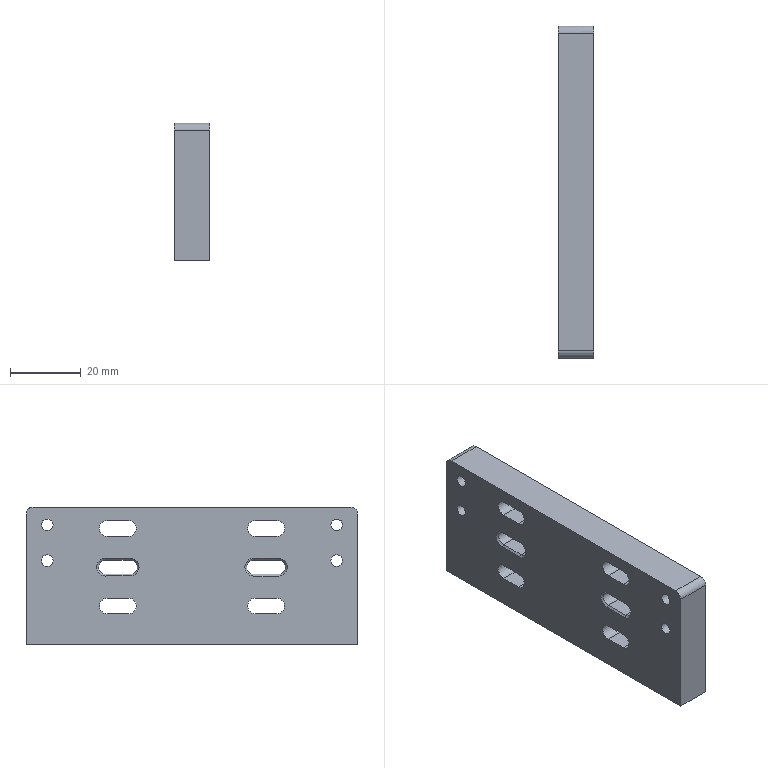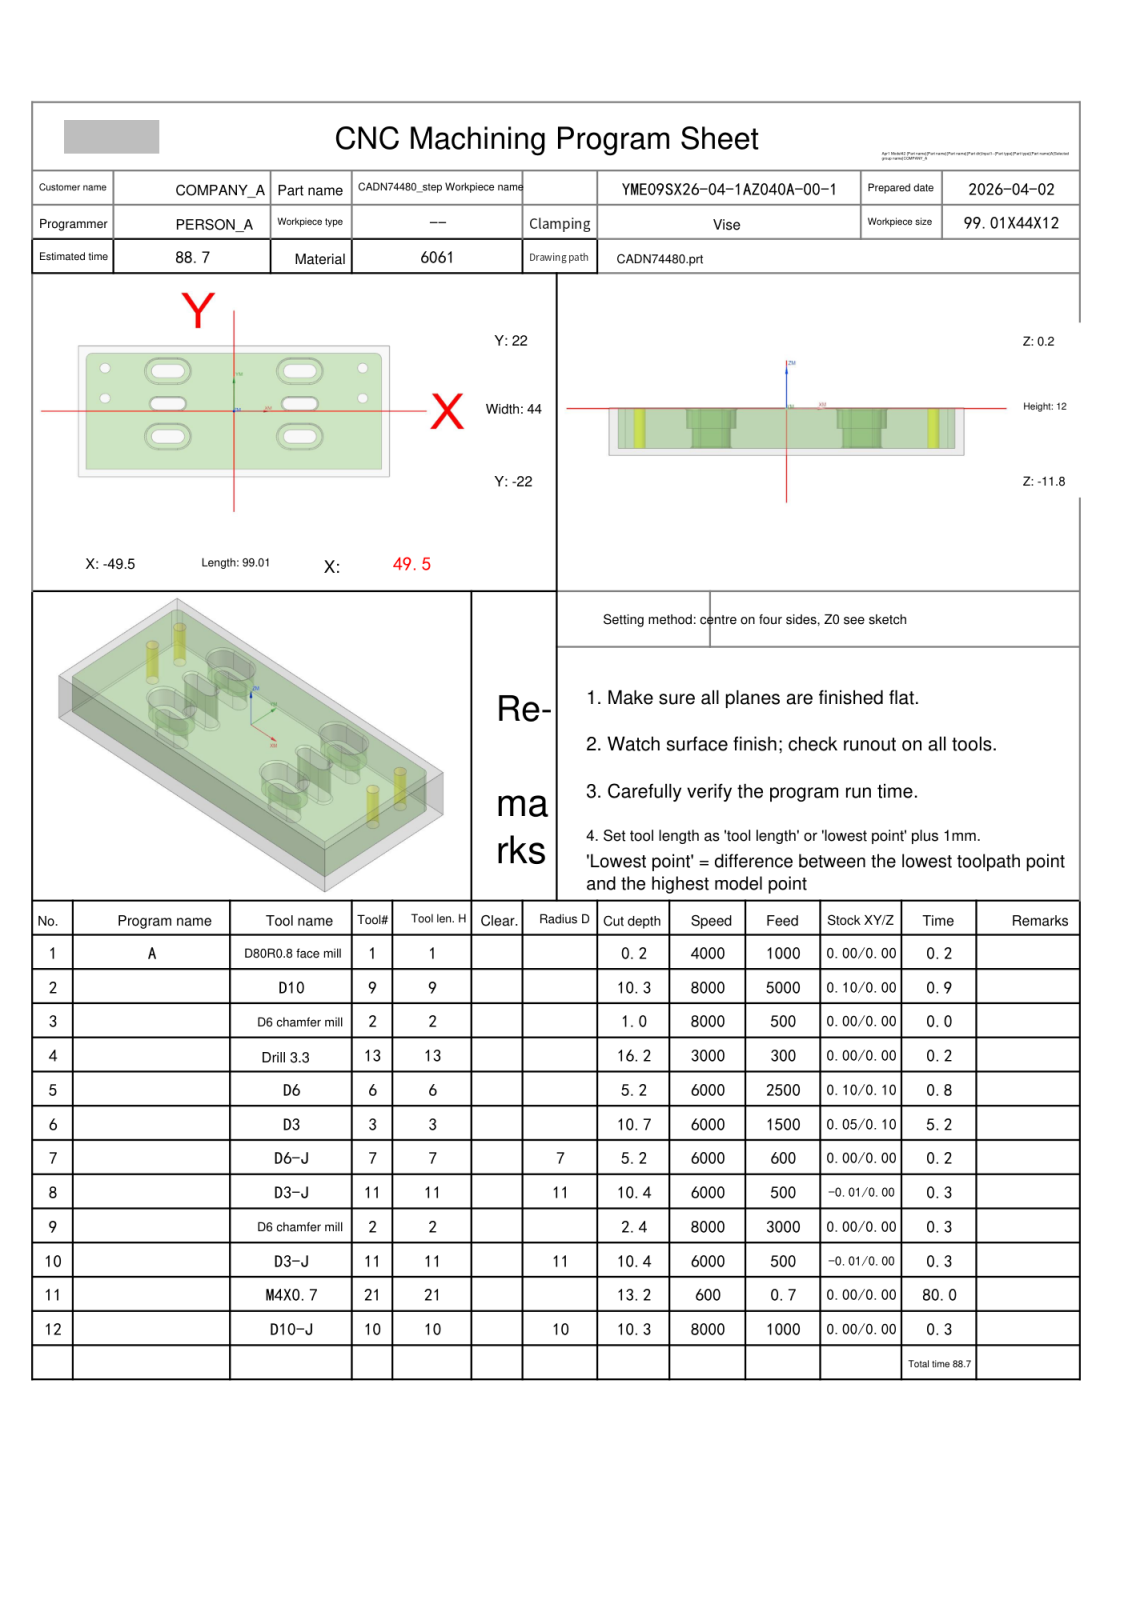NC program | NX | posted by the shop | part box 10.067 x 94 x 39 mm
Lines 938 to 1774 of 4590:
N6 T03 M06
(D3  D=3. R=0. H=03 ce=0.05 di=0.10)
G00 G90 G54 X21.004 Y-9.2 M03 S6000
G43 H03 Z20.
M08
Z-4.5
G01 X24.004 Z-4.518 F1500.
G03 X24.704 Y-8.5 Z-4.525 I0.0 J.7
X24.004 Y-7.8 Z-4.532 I-.7 J0.0
G01 X18.004 Z-4.568
G03 X17.304 Y-8.5 Z-4.575 I0.0 J-.7
X18.004 Y-9.2 Z-4.582 I.7 J0.0
G01 X24.004 Z-4.618
G03 X24.704 Y-8.5 Z-4.625 I0.0 J.7
X24.004 Y-7.8 Z-4.632 I-.7 J0.0
G01 X18.004 Z-4.668
G03 X17.304 Y-8.5 Z-4.675 I0.0 J-.7
X18.004 Y-9.2 Z-4.682 I.7 J0.0
G01 X24.004 Z-4.718
G03 X24.704 Y-8.5 Z-4.725 I0.0 J.7
X24.004 Y-7.8 Z-4.732 I-.7 J0.0
G01 X18.004 Z-4.768
G03 X17.304 Y-8.5 Z-4.775 I0.0 J-.7
X18.004 Y-9.2 Z-4.782 I.7 J0.0
G01 X24.004 Z-4.818
G03 X24.704 Y-8.5 Z-4.825 I0.0 J.7
X24.004 Y-7.8 Z-4.832 I-.7 J0.0
G01 X18.004 Z-4.868
G03 X17.304 Y-8.5 Z-4.875 I0.0 J-.7
X18.004 Y-9.2 Z-4.882 I.7 J0.0
G01 X24.004 Z-4.918
G03 X24.704 Y-8.5 Z-4.925 I0.0 J.7
X24.004 Y-7.8 Z-4.932 I-.7 J0.0
G01 X18.004 Z-4.968
G03 X17.304 Y-8.5 Z-4.975 I0.0 J-.7
X18.004 Y-9.2 Z-4.982 I.7 J0.0
G01 X24.004 Z-5.018
G03 X24.704 Y-8.5 Z-5.025 I0.0 J.7
X24.004 Y-7.8 Z-5.032 I-.7 J0.0
G01 X18.004 Z-5.068
G03 X17.304 Y-8.5 Z-5.075 I0.0 J-.7
X18.004 Y-9.2 Z-5.082 I.7 J0.0
G01 X24.004 Z-5.118
G03 X24.704 Y-8.5 Z-5.125 I0.0 J.7
X24.004 Y-7.8 Z-5.132 I-.7 J0.0
G01 X18.004 Z-5.168
G03 X17.304 Y-8.5 Z-5.175 I0.0 J-.7
X18.004 Y-9.2 Z-5.182 I.7 J0.0
G01 X24.004 Z-5.218
G03 X24.704 Y-8.5 Z-5.225 I0.0 J.7
X24.004 Y-7.8 Z-5.232 I-.7 J0.0
G01 X18.004 Z-5.268
G03 X17.304 Y-8.5 Z-5.275 I0.0 J-.7
X18.004 Y-9.2 Z-5.282 I.7 J0.0
G01 X24.004 Z-5.318
G03 X24.704 Y-8.5 Z-5.325 I0.0 J.7
X24.004 Y-7.8 Z-5.332 I-.7 J0.0
G01 X18.004 Z-5.368
G03 X17.304 Y-8.5 Z-5.375 I0.0 J-.7
X18.004 Y-9.2 Z-5.382 I.7 J0.0
G01 X24.004 Z-5.418
G03 X24.704 Y-8.5 Z-5.425 I0.0 J.7
X24.004 Y-7.8 Z-5.432 I-.7 J0.0
G01 X18.004 Z-5.468
G03 X17.304 Y-8.5 Z-5.475 I0.0 J-.7
X18.004 Y-9.2 Z-5.482 I.7 J0.0
G01 X24.004 Z-5.518
G03 X24.704 Y-8.5 Z-5.525 I0.0 J.7
X24.004 Y-7.8 Z-5.532 I-.7 J0.0
G01 X18.004 Z-5.568
G03 X17.304 Y-8.5 Z-5.575 I0.0 J-.7
X18.004 Y-9.2 Z-5.582 I.7 J0.0
G01 X24.004 Z-5.618
G03 X24.704 Y-8.5 Z-5.625 I0.0 J.7
X24.004 Y-7.8 Z-5.632 I-.7 J0.0
G01 X18.004 Z-5.668
G03 X17.304 Y-8.5 Z-5.675 I0.0 J-.7
X18.004 Y-9.2 Z-5.682 I.7 J0.0
G01 X24.004 Z-5.718
G03 X24.704 Y-8.5 Z-5.725 I0.0 J.7
X24.004 Y-7.8 Z-5.732 I-.7 J0.0
G01 X18.004 Z-5.768
G03 X17.304 Y-8.5 Z-5.775 I0.0 J-.7
X18.004 Y-9.2 Z-5.782 I.7 J0.0
G01 X24.004 Z-5.818
G03 X24.704 Y-8.5 Z-5.825 I0.0 J.7
X24.004 Y-7.8 Z-5.832 I-.7 J0.0
G01 X18.004 Z-5.868
G03 X17.304 Y-8.5 Z-5.875 I0.0 J-.7
X18.004 Y-9.2 Z-5.882 I.7 J0.0
G01 X24.004 Z-5.918
G03 X24.704 Y-8.5 Z-5.925 I0.0 J.7
X24.004 Y-7.8 Z-5.932 I-.7 J0.0
G01 X18.004 Z-5.968
G03 X17.304 Y-8.5 Z-5.975 I0.0 J-.7
X18.004 Y-9.2 Z-5.982 I.7 J0.0
G01 X24.004 Z-6.018
G03 X24.704 Y-8.5 Z-6.025 I0.0 J.7
X24.004 Y-7.8 Z-6.032 I-.7 J0.0
G01 X18.004 Z-6.068
G03 X17.304 Y-8.5 Z-6.075 I0.0 J-.7
X18.004 Y-9.2 Z-6.082 I.7 J0.0
G01 X24.004 Z-6.118
G03 X24.704 Y-8.5 Z-6.125 I0.0 J.7
X24.004 Y-7.8 Z-6.132 I-.7 J0.0
G01 X18.004 Z-6.168
G03 X17.304 Y-8.5 Z-6.175 I0.0 J-.7
X18.004 Y-9.2 Z-6.182 I.7 J0.0
G01 X24.004 Z-6.218
G03 X24.704 Y-8.5 Z-6.225 I0.0 J.7
X24.004 Y-7.8 Z-6.232 I-.7 J0.0
G01 X18.004 Z-6.268
G03 X17.304 Y-8.5 Z-6.275 I0.0 J-.7
X18.004 Y-9.2 Z-6.282 I.7 J0.0
G01 X24.004 Z-6.318
G03 X24.704 Y-8.5 Z-6.325 I0.0 J.7
X24.004 Y-7.8 Z-6.332 I-.7 J0.0
G01 X18.004 Z-6.368
G03 X17.304 Y-8.5 Z-6.375 I0.0 J-.7
X18.004 Y-9.2 Z-6.382 I.7 J0.0
G01 X24.004 Z-6.418
G03 X24.704 Y-8.5 Z-6.425 I0.0 J.7
X24.004 Y-7.8 Z-6.432 I-.7 J0.0
G01 X18.004 Z-6.468
G03 X17.304 Y-8.5 Z-6.475 I0.0 J-.7
X18.004 Y-9.2 Z-6.482 I.7 J0.0
G01 X24.004 Z-6.518
G03 X24.704 Y-8.5 Z-6.525 I0.0 J.7
X24.004 Y-7.8 Z-6.532 I-.7 J0.0
G01 X18.004 Z-6.568
G03 X17.304 Y-8.5 Z-6.575 I0.0 J-.7
X18.004 Y-9.2 Z-6.582 I.7 J0.0
G01 X24.004 Z-6.618
G03 X24.704 Y-8.5 Z-6.625 I0.0 J.7
X24.004 Y-7.8 Z-6.632 I-.7 J0.0
G01 X18.004 Z-6.668
G03 X17.304 Y-8.5 Z-6.675 I0.0 J-.7
X18.004 Y-9.2 Z-6.682 I.7 J0.0
G01 X24.004 Z-6.718
G03 X24.704 Y-8.5 Z-6.725 I0.0 J.7
X24.004 Y-7.8 Z-6.732 I-.7 J0.0
G01 X18.004 Z-6.768
G03 X17.304 Y-8.5 Z-6.775 I0.0 J-.7
X18.004 Y-9.2 Z-6.782 I.7 J0.0
G01 X24.004 Z-6.818
G03 X24.704 Y-8.5 Z-6.825 I0.0 J.7
X24.004 Y-7.8 Z-6.832 I-.7 J0.0
G01 X18.004 Z-6.868
G03 X17.304 Y-8.5 Z-6.875 I0.0 J-.7
X18.004 Y-9.2 Z-6.882 I.7 J0.0
G01 X24.004 Z-6.918
G03 X24.704 Y-8.5 Z-6.925 I0.0 J.7
X24.004 Y-7.8 Z-6.932 I-.7 J0.0
G01 X18.004 Z-6.968
G03 X17.304 Y-8.5 Z-6.975 I0.0 J-.7
X18.004 Y-9.2 Z-6.982 I.7 J0.0
G01 X24.004 Z-7.018
G03 X24.704 Y-8.5 Z-7.025 I0.0 J.7
X24.004 Y-7.8 Z-7.032 I-.7 J0.0
G01 X18.004 Z-7.068
G03 X17.304 Y-8.5 Z-7.075 I0.0 J-.7
X18.004 Y-9.2 Z-7.082 I.7 J0.0
G01 X24.004 Z-7.118
G03 X24.704 Y-8.5 Z-7.125 I0.0 J.7
X24.004 Y-7.8 Z-7.132 I-.7 J0.0
G01 X18.004 Z-7.168
G03 X17.304 Y-8.5 Z-7.175 I0.0 J-.7
X18.004 Y-9.2 Z-7.182 I.7 J0.0
G01 X24.004 Z-7.218
G03 X24.704 Y-8.5 Z-7.225 I0.0 J.7
X24.004 Y-7.8 Z-7.232 I-.7 J0.0
G01 X18.004 Z-7.268
G03 X17.304 Y-8.5 Z-7.275 I0.0 J-.7
X18.004 Y-9.2 Z-7.282 I.7 J0.0
G01 X24.004 Z-7.318
G03 X24.704 Y-8.5 Z-7.325 I0.0 J.7
X24.004 Y-7.8 Z-7.332 I-.7 J0.0
G01 X18.004 Z-7.368
G03 X17.304 Y-8.5 Z-7.375 I0.0 J-.7
X18.004 Y-9.2 Z-7.382 I.7 J0.0
G01 X24.004 Z-7.418
G03 X24.704 Y-8.5 Z-7.425 I0.0 J.7
X24.004 Y-7.8 Z-7.432 I-.7 J0.0
G01 X18.004 Z-7.468
G03 X17.304 Y-8.5 Z-7.475 I0.0 J-.7
X18.004 Y-9.2 Z-7.482 I.7 J0.0
G01 X24.004 Z-7.518
G03 X24.704 Y-8.5 Z-7.525 I0.0 J.7
X24.004 Y-7.8 Z-7.532 I-.7 J0.0
G01 X18.004 Z-7.568
G03 X17.304 Y-8.5 Z-7.575 I0.0 J-.7
X18.004 Y-9.2 Z-7.582 I.7 J0.0
G01 X24.004 Z-7.618
G03 X24.704 Y-8.5 Z-7.625 I0.0 J.7
X24.004 Y-7.8 Z-7.632 I-.7 J0.0
G01 X18.004 Z-7.668
G03 X17.304 Y-8.5 Z-7.675 I0.0 J-.7
X18.004 Y-9.2 Z-7.682 I.7 J0.0
G01 X24.004 Z-7.718
G03 X24.704 Y-8.5 Z-7.725 I0.0 J.7
X24.004 Y-7.8 Z-7.732 I-.7 J0.0
G01 X18.004 Z-7.768
G03 X17.304 Y-8.5 Z-7.775 I0.0 J-.7
X18.004 Y-9.2 Z-7.782 I.7 J0.0
G01 X24.004 Z-7.818
G03 X24.704 Y-8.5 Z-7.825 I0.0 J.7
X24.004 Y-7.8 Z-7.832 I-.7 J0.0
G01 X18.004 Z-7.868
G03 X17.304 Y-8.5 Z-7.875 I0.0 J-.7
X18.004 Y-9.2 Z-7.882 I.7 J0.0
G01 X24.004 Z-7.918
G03 X24.704 Y-8.5 Z-7.925 I0.0 J.7
X24.004 Y-7.8 Z-7.932 I-.7 J0.0
G01 X18.004 Z-7.968
G03 X17.304 Y-8.5 Z-7.975 I0.0 J-.7
X18.004 Y-9.2 Z-7.982 I.7 J0.0
G01 X24.004 Z-8.018
G03 X24.704 Y-8.5 Z-8.025 I0.0 J.7
X24.004 Y-7.8 Z-8.032 I-.7 J0.0
G01 X18.004 Z-8.068
G03 X17.304 Y-8.5 Z-8.075 I0.0 J-.7
X18.004 Y-9.2 Z-8.082 I.7 J0.0
G01 X24.004 Z-8.118
G03 X24.704 Y-8.5 Z-8.125 I0.0 J.7
X24.004 Y-7.8 Z-8.132 I-.7 J0.0
G01 X18.004 Z-8.168
G03 X17.304 Y-8.5 Z-8.175 I0.0 J-.7
X18.004 Y-9.2 Z-8.182 I.7 J0.0
G01 X24.004 Z-8.218
G03 X24.704 Y-8.5 Z-8.225 I0.0 J.7
X24.004 Y-7.8 Z-8.232 I-.7 J0.0
G01 X18.004 Z-8.268
G03 X17.304 Y-8.5 Z-8.275 I0.0 J-.7
X18.004 Y-9.2 Z-8.282 I.7 J0.0
G01 X24.004 Z-8.318
G03 X24.704 Y-8.5 Z-8.325 I0.0 J.7
X24.004 Y-7.8 Z-8.332 I-.7 J0.0
G01 X18.004 Z-8.368
G03 X17.304 Y-8.5 Z-8.375 I0.0 J-.7
X18.004 Y-9.2 Z-8.382 I.7 J0.0
G01 X24.004 Z-8.418
G03 X24.704 Y-8.5 Z-8.425 I0.0 J.7
X24.004 Y-7.8 Z-8.432 I-.7 J0.0
G01 X18.004 Z-8.468
G03 X17.304 Y-8.5 Z-8.475 I0.0 J-.7
X18.004 Y-9.2 Z-8.482 I.7 J0.0
G01 X24.004 Z-8.518
G03 X24.704 Y-8.5 Z-8.525 I0.0 J.7
X24.004 Y-7.8 Z-8.532 I-.7 J0.0
G01 X18.004 Z-8.568
G03 X17.304 Y-8.5 Z-8.575 I0.0 J-.7
X18.004 Y-9.2 Z-8.582 I.7 J0.0
G01 X24.004 Z-8.618
G03 X24.704 Y-8.5 Z-8.625 I0.0 J.7
X24.004 Y-7.8 Z-8.632 I-.7 J0.0
G01 X18.004 Z-8.668
G03 X17.304 Y-8.5 Z-8.675 I0.0 J-.7
X18.004 Y-9.2 Z-8.682 I.7 J0.0
G01 X24.004 Z-8.718
G03 X24.704 Y-8.5 Z-8.725 I0.0 J.7
X24.004 Y-7.8 Z-8.732 I-.7 J0.0
G01 X18.004 Z-8.768
G03 X17.304 Y-8.5 Z-8.775 I0.0 J-.7
X18.004 Y-9.2 Z-8.782 I.7 J0.0
G01 X24.004 Z-8.818
G03 X24.704 Y-8.5 Z-8.825 I0.0 J.7
X24.004 Y-7.8 Z-8.832 I-.7 J0.0
G01 X18.004 Z-8.868
G03 X17.304 Y-8.5 Z-8.875 I0.0 J-.7
X18.004 Y-9.2 Z-8.882 I.7 J0.0
G01 X24.004 Z-8.918
G03 X24.704 Y-8.5 Z-8.925 I0.0 J.7
X24.004 Y-7.8 Z-8.932 I-.7 J0.0
G01 X18.004 Z-8.968
G03 X17.304 Y-8.5 Z-8.975 I0.0 J-.7
X18.004 Y-9.2 Z-8.982 I.7 J0.0
G01 X24.004 Z-9.018
G03 X24.704 Y-8.5 Z-9.025 I0.0 J.7
X24.004 Y-7.8 Z-9.032 I-.7 J0.0
G01 X18.004 Z-9.068
G03 X17.304 Y-8.5 Z-9.075 I0.0 J-.7
X18.004 Y-9.2 Z-9.082 I.7 J0.0
G01 X24.004 Z-9.118
G03 X24.704 Y-8.5 Z-9.125 I0.0 J.7
X24.004 Y-7.8 Z-9.132 I-.7 J0.0
G01 X18.004 Z-9.168
G03 X17.304 Y-8.5 Z-9.175 I0.0 J-.7
X18.004 Y-9.2 Z-9.182 I.7 J0.0
G01 X24.004 Z-9.218
G03 X24.704 Y-8.5 Z-9.225 I0.0 J.7
X24.004 Y-7.8 Z-9.232 I-.7 J0.0
G01 X18.004 Z-9.268
G03 X17.304 Y-8.5 Z-9.275 I0.0 J-.7
X18.004 Y-9.2 Z-9.282 I.7 J0.0
G01 X24.004 Z-9.318
G03 X24.704 Y-8.5 Z-9.325 I0.0 J.7
X24.004 Y-7.8 Z-9.332 I-.7 J0.0
G01 X18.004 Z-9.368
G03 X17.304 Y-8.5 Z-9.375 I0.0 J-.7
X18.004 Y-9.2 Z-9.382 I.7 J0.0
G01 X24.004 Z-9.418
G03 X24.704 Y-8.5 Z-9.425 I0.0 J.7
X24.004 Y-7.8 Z-9.432 I-.7 J0.0
G01 X18.004 Z-9.468
G03 X17.304 Y-8.5 Z-9.475 I0.0 J-.7
X18.004 Y-9.2 Z-9.482 I.7 J0.0
G01 X24.004 Z-9.518
G03 X24.704 Y-8.5 Z-9.525 I0.0 J.7
X24.004 Y-7.8 Z-9.532 I-.7 J0.0
G01 X18.004 Z-9.568
G03 X17.304 Y-8.5 Z-9.575 I0.0 J-.7
X18.004 Y-9.2 Z-9.582 I.7 J0.0
G01 X24.004 Z-9.618
G03 X24.704 Y-8.5 Z-9.625 I0.0 J.7
X24.004 Y-7.8 Z-9.632 I-.7 J0.0
G01 X18.004 Z-9.668
G03 X17.304 Y-8.5 Z-9.675 I0.0 J-.7
X18.004 Y-9.2 Z-9.682 I.7 J0.0
G01 X24.004 Z-9.718
G03 X24.704 Y-8.5 Z-9.725 I0.0 J.7
X24.004 Y-7.8 Z-9.732 I-.7 J0.0
G01 X18.004 Z-9.768
G03 X17.304 Y-8.5 Z-9.775 I0.0 J-.7
X18.004 Y-9.2 Z-9.782 I.7 J0.0
G01 X24.004 Z-9.818
G03 X24.704 Y-8.5 Z-9.825 I0.0 J.7
X24.004 Y-7.8 Z-9.832 I-.7 J0.0
G01 X18.004 Z-9.868
G03 X17.304 Y-8.5 Z-9.875 I0.0 J-.7
X18.004 Y-9.2 Z-9.882 I.7 J0.0
G01 X24.004 Z-9.918
G03 X24.704 Y-8.5 Z-9.925 I0.0 J.7
X24.004 Y-7.8 Z-9.932 I-.7 J0.0
G01 X18.004 Z-9.968
G03 X17.304 Y-8.5 Z-9.975 I0.0 J-.7
X18.004 Y-9.2 Z-9.982 I.7 J0.0
G01 X24.004 Z-10.018
G03 X24.704 Y-8.5 Z-10.025 I0.0 J.7
X24.004 Y-7.8 Z-10.032 I-.7 J0.0
G01 X18.004 Z-10.068
G03 X17.304 Y-8.5 Z-10.075 I0.0 J-.7
X18.004 Y-9.2 Z-10.082 I.7 J0.0
G01 X24.004 Z-10.118
G03 X24.704 Y-8.5 Z-10.125 I0.0 J.7
X24.004 Y-7.8 Z-10.132 I-.7 J0.0
G01 X18.004 Z-10.168
G03 X17.304 Y-8.5 Z-10.175 I0.0 J-.7
X18.004 Y-9.2 Z-10.182 I.7 J0.0
G01 X24.004 Z-10.218
G03 X24.704 Y-8.5 Z-10.225 I0.0 J.7
X24.004 Y-7.8 Z-10.232 I-.7 J0.0
G01 X18.004 Z-10.268
G03 X17.304 Y-8.5 Z-10.275 I0.0 J-.7
X18.004 Y-9.2 Z-10.282 I.7 J0.0
G01 X24.004 Z-10.318
G03 X24.704 Y-8.5 Z-10.325 I0.0 J.7
X24.004 Y-7.8 Z-10.332 I-.7 J0.0
G01 X18.004 Z-10.368
G03 X17.304 Y-8.5 Z-10.375 I0.0 J-.7
X18.004 Y-9.2 Z-10.382 I.7 J0.0
G01 X24.004 Z-10.418
G03 X24.704 Y-8.5 Z-10.425 I0.0 J.7
X24.004 Y-7.8 Z-10.432 I-.7 J0.0
G01 X18.004 Z-10.468
G03 X17.304 Y-8.5 Z-10.475 I0.0 J-.7
X18.004 Y-9.2 Z-10.482 I.7 J0.0
G01 X21.004 Z-10.5
X24.004
G03 X24.704 Y-8.5 I0.0 J.7
X24.004 Y-7.8 I-.7 J0.0
G01 X18.004
G03 X17.304 Y-8.5 I0.0 J-.7
X18.004 Y-9.2 I.7 J0.0
G01 X21.004
X21.504
Z-9.5
G00 Z20.
X21.004 Y14.2
Z-4.5
G01 X18.004 Z-4.518
G03 X17.304 Y13.5 Z-4.525 I0.0 J-.7
X18.004 Y12.8 Z-4.532 I.7 J0.0
G01 X24.004 Z-4.568
G03 X24.704 Y13.5 Z-4.575 I0.0 J.7
X24.004 Y14.2 Z-4.582 I-.7 J0.0
G01 X18.004 Z-4.618
G03 X17.304 Y13.5 Z-4.625 I0.0 J-.7
X18.004 Y12.8 Z-4.632 I.7 J0.0
G01 X24.004 Z-4.668
G03 X24.704 Y13.5 Z-4.675 I0.0 J.7
X24.004 Y14.2 Z-4.682 I-.7 J0.0
G01 X18.004 Z-4.718
G03 X17.304 Y13.5 Z-4.725 I0.0 J-.7
X18.004 Y12.8 Z-4.732 I.7 J0.0
G01 X24.004 Z-4.768
G03 X24.704 Y13.5 Z-4.775 I0.0 J.7
X24.004 Y14.2 Z-4.782 I-.7 J0.0
G01 X18.004 Z-4.818
G03 X17.304 Y13.5 Z-4.825 I0.0 J-.7
X18.004 Y12.8 Z-4.832 I.7 J0.0
G01 X24.004 Z-4.868
G03 X24.704 Y13.5 Z-4.875 I0.0 J.7
X24.004 Y14.2 Z-4.882 I-.7 J0.0
G01 X18.004 Z-4.918
G03 X17.304 Y13.5 Z-4.925 I0.0 J-.7
X18.004 Y12.8 Z-4.932 I.7 J0.0
G01 X24.004 Z-4.968
G03 X24.704 Y13.5 Z-4.975 I0.0 J.7
X24.004 Y14.2 Z-4.982 I-.7 J0.0
G01 X18.004 Z-5.018
G03 X17.304 Y13.5 Z-5.025 I0.0 J-.7
X18.004 Y12.8 Z-5.032 I.7 J0.0
G01 X24.004 Z-5.068
G03 X24.704 Y13.5 Z-5.075 I0.0 J.7
X24.004 Y14.2 Z-5.082 I-.7 J0.0
G01 X18.004 Z-5.118
G03 X17.304 Y13.5 Z-5.125 I0.0 J-.7
X18.004 Y12.8 Z-5.132 I.7 J0.0
G01 X24.004 Z-5.168
G03 X24.704 Y13.5 Z-5.175 I0.0 J.7
X24.004 Y14.2 Z-5.182 I-.7 J0.0
G01 X18.004 Z-5.218
G03 X17.304 Y13.5 Z-5.225 I0.0 J-.7
X18.004 Y12.8 Z-5.232 I.7 J0.0
G01 X24.004 Z-5.268
G03 X24.704 Y13.5 Z-5.275 I0.0 J.7
X24.004 Y14.2 Z-5.282 I-.7 J0.0
G01 X18.004 Z-5.318
G03 X17.304 Y13.5 Z-5.325 I0.0 J-.7
X18.004 Y12.8 Z-5.332 I.7 J0.0
G01 X24.004 Z-5.368
G03 X24.704 Y13.5 Z-5.375 I0.0 J.7
X24.004 Y14.2 Z-5.382 I-.7 J0.0
G01 X18.004 Z-5.418
G03 X17.304 Y13.5 Z-5.425 I0.0 J-.7
X18.004 Y12.8 Z-5.432 I.7 J0.0
G01 X24.004 Z-5.468
G03 X24.704 Y13.5 Z-5.475 I0.0 J.7
X24.004 Y14.2 Z-5.482 I-.7 J0.0
G01 X18.004 Z-5.518
G03 X17.304 Y13.5 Z-5.525 I0.0 J-.7
X18.004 Y12.8 Z-5.532 I.7 J0.0
G01 X24.004 Z-5.568
G03 X24.704 Y13.5 Z-5.575 I0.0 J.7
X24.004 Y14.2 Z-5.582 I-.7 J0.0
G01 X18.004 Z-5.618
G03 X17.304 Y13.5 Z-5.625 I0.0 J-.7
X18.004 Y12.8 Z-5.632 I.7 J0.0
G01 X24.004 Z-5.668
G03 X24.704 Y13.5 Z-5.675 I0.0 J.7
X24.004 Y14.2 Z-5.682 I-.7 J0.0
G01 X18.004 Z-5.718
G03 X17.304 Y13.5 Z-5.725 I0.0 J-.7
X18.004 Y12.8 Z-5.732 I.7 J0.0
G01 X24.004 Z-5.768
G03 X24.704 Y13.5 Z-5.775 I0.0 J.7
X24.004 Y14.2 Z-5.782 I-.7 J0.0
G01 X18.004 Z-5.818
G03 X17.304 Y13.5 Z-5.825 I0.0 J-.7
X18.004 Y12.8 Z-5.832 I.7 J0.0
G01 X24.004 Z-5.868
G03 X24.704 Y13.5 Z-5.875 I0.0 J.7
X24.004 Y14.2 Z-5.882 I-.7 J0.0
G01 X18.004 Z-5.918
G03 X17.304 Y13.5 Z-5.925 I0.0 J-.7
X18.004 Y12.8 Z-5.932 I.7 J0.0
G01 X24.004 Z-5.968
G03 X24.704 Y13.5 Z-5.975 I0.0 J.7
X24.004 Y14.2 Z-5.982 I-.7 J0.0
G01 X18.004 Z-6.018
G03 X17.304 Y13.5 Z-6.025 I0.0 J-.7
X18.004 Y12.8 Z-6.032 I.7 J0.0
G01 X24.004 Z-6.068
G03 X24.704 Y13.5 Z-6.075 I0.0 J.7
X24.004 Y14.2 Z-6.082 I-.7 J0.0
G01 X18.004 Z-6.118
G03 X17.304 Y13.5 Z-6.125 I0.0 J-.7
X18.004 Y12.8 Z-6.132 I.7 J0.0
G01 X24.004 Z-6.168
G03 X24.704 Y13.5 Z-6.175 I0.0 J.7
X24.004 Y14.2 Z-6.182 I-.7 J0.0
G01 X18.004 Z-6.218
G03 X17.304 Y13.5 Z-6.225 I0.0 J-.7
X18.004 Y12.8 Z-6.232 I.7 J0.0
G01 X24.004 Z-6.268
G03 X24.704 Y13.5 Z-6.275 I0.0 J.7
X24.004 Y14.2 Z-6.282 I-.7 J0.0
G01 X18.004 Z-6.318
G03 X17.304 Y13.5 Z-6.325 I0.0 J-.7
X18.004 Y12.8 Z-6.332 I.7 J0.0
G01 X24.004 Z-6.368
G03 X24.704 Y13.5 Z-6.375 I0.0 J.7
X24.004 Y14.2 Z-6.382 I-.7 J0.0
G01 X18.004 Z-6.418
G03 X17.304 Y13.5 Z-6.425 I0.0 J-.7
X18.004 Y12.8 Z-6.432 I.7 J0.0
G01 X24.004 Z-6.468
G03 X24.704 Y13.5 Z-6.475 I0.0 J.7
X24.004 Y14.2 Z-6.482 I-.7 J0.0
G01 X18.004 Z-6.518
G03 X17.304 Y13.5 Z-6.525 I0.0 J-.7
X18.004 Y12.8 Z-6.532 I.7 J0.0
G01 X24.004 Z-6.568
G03 X24.704 Y13.5 Z-6.575 I0.0 J.7
X24.004 Y14.2 Z-6.582 I-.7 J0.0
G01 X18.004 Z-6.618
G03 X17.304 Y13.5 Z-6.625 I0.0 J-.7
X18.004 Y12.8 Z-6.632 I.7 J0.0
G01 X24.004 Z-6.668
G03 X24.704 Y13.5 Z-6.675 I0.0 J.7
X24.004 Y14.2 Z-6.682 I-.7 J0.0
G01 X18.004 Z-6.718
G03 X17.304 Y13.5 Z-6.725 I0.0 J-.7
X18.004 Y12.8 Z-6.732 I.7 J0.0
G01 X24.004 Z-6.768
G03 X24.704 Y13.5 Z-6.775 I0.0 J.7
X24.004 Y14.2 Z-6.782 I-.7 J0.0
G01 X18.004 Z-6.818
G03 X17.304 Y13.5 Z-6.825 I0.0 J-.7
X18.004 Y12.8 Z-6.832 I.7 J0.0
G01 X24.004 Z-6.868
G03 X24.704 Y13.5 Z-6.875 I0.0 J.7
X24.004 Y14.2 Z-6.882 I-.7 J0.0
G01 X18.004 Z-6.918
G03 X17.304 Y13.5 Z-6.925 I0.0 J-.7
X18.004 Y12.8 Z-6.932 I.7 J0.0
G01 X24.004 Z-6.968
G03 X24.704 Y13.5 Z-6.975 I0.0 J.7
X24.004 Y14.2 Z-6.982 I-.7 J0.0
G01 X18.004 Z-7.018
G03 X17.304 Y13.5 Z-7.025 I0.0 J-.7
X18.004 Y12.8 Z-7.032 I.7 J0.0
G01 X24.004 Z-7.068
G03 X24.704 Y13.5 Z-7.075 I0.0 J.7
X24.004 Y14.2 Z-7.082 I-.7 J0.0
G01 X18.004 Z-7.118
G03 X17.304 Y13.5 Z-7.125 I0.0 J-.7
X18.004 Y12.8 Z-7.132 I.7 J0.0
G01 X24.004 Z-7.168
G03 X24.704 Y13.5 Z-7.175 I0.0 J.7
X24.004 Y14.2 Z-7.182 I-.7 J0.0
G01 X18.004 Z-7.218
G03 X17.304 Y13.5 Z-7.225 I0.0 J-.7
X18.004 Y12.8 Z-7.232 I.7 J0.0
G01 X24.004 Z-7.268
G03 X24.704 Y13.5 Z-7.275 I0.0 J.7
X24.004 Y14.2 Z-7.282 I-.7 J0.0
G01 X18.004 Z-7.318
G03 X17.304 Y13.5 Z-7.325 I0.0 J-.7
X18.004 Y12.8 Z-7.332 I.7 J0.0
G01 X24.004 Z-7.368
G03 X24.704 Y13.5 Z-7.375 I0.0 J.7
X24.004 Y14.2 Z-7.382 I-.7 J0.0
G01 X18.004 Z-7.418
G03 X17.304 Y13.5 Z-7.425 I0.0 J-.7
X18.004 Y12.8 Z-7.432 I.7 J0.0
G01 X24.004 Z-7.468
G03 X24.704 Y13.5 Z-7.475 I0.0 J.7
X24.004 Y14.2 Z-7.482 I-.7 J0.0
G01 X18.004 Z-7.518
G03 X17.304 Y13.5 Z-7.525 I0.0 J-.7
X18.004 Y12.8 Z-7.532 I.7 J0.0
G01 X24.004 Z-7.568
G03 X24.704 Y13.5 Z-7.575 I0.0 J.7
X24.004 Y14.2 Z-7.582 I-.7 J0.0
G01 X18.004 Z-7.618
G03 X17.304 Y13.5 Z-7.625 I0.0 J-.7
X18.004 Y12.8 Z-7.632 I.7 J0.0
G01 X24.004 Z-7.668
G03 X24.704 Y13.5 Z-7.675 I0.0 J.7
X24.004 Y14.2 Z-7.682 I-.7 J0.0
G01 X18.004 Z-7.718
G03 X17.304 Y13.5 Z-7.725 I0.0 J-.7
X18.004 Y12.8 Z-7.732 I.7 J0.0
G01 X24.004 Z-7.768
G03 X24.704 Y13.5 Z-7.775 I0.0 J.7
X24.004 Y14.2 Z-7.782 I-.7 J0.0
G01 X18.004 Z-7.818
G03 X17.304 Y13.5 Z-7.825 I0.0 J-.7
X18.004 Y12.8 Z-7.832 I.7 J0.0
G01 X24.004 Z-7.868
G03 X24.704 Y13.5 Z-7.875 I0.0 J.7
X24.004 Y14.2 Z-7.882 I-.7 J0.0
G01 X18.004 Z-7.918
G03 X17.304 Y13.5 Z-7.925 I0.0 J-.7
X18.004 Y12.8 Z-7.932 I.7 J0.0
G01 X24.004 Z-7.968
G03 X24.704 Y13.5 Z-7.975 I0.0 J.7
X24.004 Y14.2 Z-7.982 I-.7 J0.0
G01 X18.004 Z-8.018
G03 X17.304 Y13.5 Z-8.025 I0.0 J-.7
X18.004 Y12.8 Z-8.032 I.7 J0.0
G01 X24.004 Z-8.068
G03 X24.704 Y13.5 Z-8.075 I0.0 J.7
X24.004 Y14.2 Z-8.082 I-.7 J0.0
G01 X18.004 Z-8.118
G03 X17.304 Y13.5 Z-8.125 I0.0 J-.7
X18.004 Y12.8 Z-8.132 I.7 J0.0
G01 X24.004 Z-8.168
G03 X24.704 Y13.5 Z-8.175 I0.0 J.7
X24.004 Y14.2 Z-8.182 I-.7 J0.0
G01 X18.004 Z-8.218
G03 X17.304 Y13.5 Z-8.225 I0.0 J-.7
X18.004 Y12.8 Z-8.232 I.7 J0.0
G01 X24.004 Z-8.268
G03 X24.704 Y13.5 Z-8.275 I0.0 J.7
X24.004 Y14.2 Z-8.282 I-.7 J0.0
G01 X18.004 Z-8.318
G03 X17.304 Y13.5 Z-8.325 I0.0 J-.7
X18.004 Y12.8 Z-8.332 I.7 J0.0
G01 X24.004 Z-8.368
G03 X24.704 Y13.5 Z-8.375 I0.0 J.7
X24.004 Y14.2 Z-8.382 I-.7 J0.0
G01 X18.004 Z-8.418
G03 X17.304 Y13.5 Z-8.425 I0.0 J-.7
X18.004 Y12.8 Z-8.432 I.7 J0.0
G01 X24.004 Z-8.468
G03 X24.704 Y13.5 Z-8.475 I0.0 J.7
X24.004 Y14.2 Z-8.482 I-.7 J0.0
G01 X18.004 Z-8.518
G03 X17.304 Y13.5 Z-8.525 I0.0 J-.7
X18.004 Y12.8 Z-8.532 I.7 J0.0
G01 X24.004 Z-8.568
G03 X24.704 Y13.5 Z-8.575 I0.0 J.7
X24.004 Y14.2 Z-8.582 I-.7 J0.0
G01 X18.004 Z-8.618
G03 X17.304 Y13.5 Z-8.625 I0.0 J-.7
X18.004 Y12.8 Z-8.632 I.7 J0.0
G01 X24.004 Z-8.668
G03 X24.704 Y13.5 Z-8.675 I0.0 J.7
X24.004 Y14.2 Z-8.682 I-.7 J0.0
G01 X18.004 Z-8.718
G03 X17.304 Y13.5 Z-8.725 I0.0 J-.7
X18.004 Y12.8 Z-8.732 I.7 J0.0
G01 X24.004 Z-8.768
G03 X24.704 Y13.5 Z-8.775 I0.0 J.7
X24.004 Y14.2 Z-8.782 I-.7 J0.0
G01 X18.004 Z-8.818
G03 X17.304 Y13.5 Z-8.825 I0.0 J-.7
X18.004 Y12.8 Z-8.832 I.7 J0.0
G01 X24.004 Z-8.868
G03 X24.704 Y13.5 Z-8.875 I0.0 J.7
X24.004 Y14.2 Z-8.882 I-.7 J0.0
G01 X18.004 Z-8.918
G03 X17.304 Y13.5 Z-8.925 I0.0 J-.7
X18.004 Y12.8 Z-8.932 I.7 J0.0
G01 X24.004 Z-8.968
G03 X24.704 Y13.5 Z-8.975 I0.0 J.7
X24.004 Y14.2 Z-8.982 I-.7 J0.0
G01 X18.004 Z-9.018
G03 X17.304 Y13.5 Z-9.025 I0.0 J-.7
X18.004 Y12.8 Z-9.032 I.7 J0.0
G01 X24.004 Z-9.068
G03 X24.704 Y13.5 Z-9.075 I0.0 J.7
X24.004 Y14.2 Z-9.082 I-.7 J0.0
G01 X18.004 Z-9.118
G03 X17.304 Y13.5 Z-9.125 I0.0 J-.7
X18.004 Y12.8 Z-9.132 I.7 J0.0
G01 X24.004 Z-9.168
G03 X24.704 Y13.5 Z-9.175 I0.0 J.7
X24.004 Y14.2 Z-9.182 I-.7 J0.0
G01 X18.004 Z-9.218
G03 X17.304 Y13.5 Z-9.225 I0.0 J-.7
X18.004 Y12.8 Z-9.232 I.7 J0.0
G01 X24.004 Z-9.268
G03 X24.704 Y13.5 Z-9.275 I0.0 J.7
X24.004 Y14.2 Z-9.282 I-.7 J0.0
G01 X18.004 Z-9.318
G03 X17.304 Y13.5 Z-9.325 I0.0 J-.7
X18.004 Y12.8 Z-9.332 I.7 J0.0
G01 X24.004 Z-9.368
G03 X24.704 Y13.5 Z-9.375 I0.0 J.7
X24.004 Y14.2 Z-9.382 I-.7 J0.0
G01 X18.004 Z-9.418
G03 X17.304 Y13.5 Z-9.425 I0.0 J-.7
X18.004 Y12.8 Z-9.432 I.7 J0.0
G01 X24.004 Z-9.468
G03 X24.704 Y13.5 Z-9.475 I0.0 J.7
X24.004 Y14.2 Z-9.482 I-.7 J0.0
G01 X18.004 Z-9.518
G03 X17.304 Y13.5 Z-9.525 I0.0 J-.7
X18.004 Y12.8 Z-9.532 I.7 J0.0
G01 X24.004 Z-9.568
G03 X24.704 Y13.5 Z-9.575 I0.0 J.7
X24.004 Y14.2 Z-9.582 I-.7 J0.0
G01 X18.004 Z-9.618
G03 X17.304 Y13.5 Z-9.625 I0.0 J-.7
X18.004 Y12.8 Z-9.632 I.7 J0.0
G01 X24.004 Z-9.668
G03 X24.704 Y13.5 Z-9.675 I0.0 J.7
X24.004 Y14.2 Z-9.682 I-.7 J0.0
G01 X18.004 Z-9.718
G03 X17.304 Y13.5 Z-9.725 I0.0 J-.7
X18.004 Y12.8 Z-9.732 I.7 J0.0
G01 X24.004 Z-9.768
G03 X24.704 Y13.5 Z-9.775 I0.0 J.7
X24.004 Y14.2 Z-9.782 I-.7 J0.0
G01 X18.004 Z-9.818
G03 X17.304 Y13.5 Z-9.825 I0.0 J-.7
X18.004 Y12.8 Z-9.832 I.7 J0.0
G01 X24.004 Z-9.868
G03 X24.704 Y13.5 Z-9.875 I0.0 J.7
X24.004 Y14.2 Z-9.882 I-.7 J0.0
G01 X18.004 Z-9.918
G03 X17.304 Y13.5 Z-9.925 I0.0 J-.7
X18.004 Y12.8 Z-9.932 I.7 J0.0
G01 X24.004 Z-9.968
G03 X24.704 Y13.5 Z-9.975 I0.0 J.7
X24.004 Y14.2 Z-9.982 I-.7 J0.0
G01 X18.004 Z-10.018
G03 X17.304 Y13.5 Z-10.025 I0.0 J-.7
X18.004 Y12.8 Z-10.032 I.7 J0.0
G01 X24.004 Z-10.068
G03 X24.704 Y13.5 Z-10.075 I0.0 J.7
X24.004 Y14.2 Z-10.082 I-.7 J0.0
G01 X18.004 Z-10.118
G03 X17.304 Y13.5 Z-10.125 I0.0 J-.7
X18.004 Y12.8 Z-10.132 I.7 J0.0
G01 X24.004 Z-10.168
G03 X24.704 Y13.5 Z-10.175 I0.0 J.7
X24.004 Y14.2 Z-10.182 I-.7 J0.0
G01 X18.004 Z-10.218
G03 X17.304 Y13.5 Z-10.225 I0.0 J-.7
X18.004 Y12.8 Z-10.232 I.7 J0.0
G01 X24.004 Z-10.268
G03 X24.704 Y13.5 Z-10.275 I0.0 J.7
X24.004 Y14.2 Z-10.282 I-.7 J0.0
G01 X18.004 Z-10.318
G03 X17.304 Y13.5 Z-10.325 I0.0 J-.7
X18.004 Y12.8 Z-10.332 I.7 J0.0
G01 X24.004 Z-10.368
G03 X24.704 Y13.5 Z-10.375 I0.0 J.7
X24.004 Y14.2 Z-10.382 I-.7 J0.0
G01 X18.004 Z-10.418
G03 X17.304 Y13.5 Z-10.425 I0.0 J-.7
X18.004 Y12.8 Z-10.432 I.7 J0.0
G01 X24.004 Z-10.468
G03 X24.704 Y13.5 Z-10.475 I0.0 J.7
X24.004 Y14.2 Z-10.482 I-.7 J0.0
G01 X21.004 Z-10.5
X18.004
G03 X17.304 Y13.5 I0.0 J-.7
X18.004 Y12.8 I.7 J0.0
G01 X24.004
G03 X24.704 Y13.5 I0.0 J.7
X24.004 Y14.2 I-.7 J0.0
G01 X21.004
X20.504
Z-9.5
G00 Z20.
X-20.996
Z-4.5
G01 X-23.996 Z-4.518
G03 X-24.696 Y13.5 Z-4.525 I0.0 J-.7
X-23.996 Y12.8 Z-4.531 I.7 J0.0
G01 X-17.996 Z-4.567
G03 X-17.296 Y13.5 Z-4.574 I0.0 J.7
X-17.996 Y14.2 Z-4.58 I-.7 J0.0
G01 X-23.996 Z-4.616
G03 X-24.696 Y13.5 Z-4.623 I0.0 J-.7
X-23.996 Y12.8 Z-4.63 I.7 J0.0
G01 X-17.996 Z-4.666
G03 X-17.296 Y13.5 Z-4.672 I0.0 J.7
X-17.996 Y14.2 Z-4.679 I-.7 J0.0
G01 X-23.996 Z-4.715
G03 X-24.696 Y13.5 Z-4.721 I0.0 J-.7
X-23.996 Y12.8 Z-4.728 I.7 J0.0
G01 X-17.996 Z-4.764
G03 X-17.296 Y13.5 Z-4.77 I0.0 J.7
X-17.996 Y14.2 Z-4.777 I-.7 J0.0
G01 X-23.996 Z-4.813
G03 X-24.696 Y13.5 Z-4.82 I0.0 J-.7
X-23.996 Y12.8 Z-4.826 I.7 J0.0
G01 X-17.996 Z-4.862
G03 X-17.296 Y13.5 Z-4.869 I0.0 J.7
X-17.996 Y14.2 Z-4.875 I-.7 J0.0
G01 X-23.996 Z-4.911
G03 X-24.696 Y13.5 Z-4.918 I0.0 J-.7
X-23.996 Y12.8 Z-4.925 I.7 J0.0
G01 X-17.996 Z-4.961
G03 X-17.296 Y13.5 Z-4.967 I0.0 J.7
X-17.996 Y14.2 Z-4.974 I-.7 J0.0
G01 X-23.996 Z-5.01
G03 X-24.696 Y13.5 Z-5.016 I0.0 J-.7
X-23.996 Y12.8 Z-5.023 I.7 J0.0
G01 X-17.996 Z-5.059
G03 X-17.296 Y13.5 Z-5.066 I0.0 J.7
X-17.996 Y14.2 Z-5.072 I-.7 J0.0
G01 X-23.996 Z-5.108
G03 X-24.696 Y13.5 Z-5.115 I0.0 J-.7
X-23.996 Y12.8 Z-5.121 I.7 J0.0
G01 X-17.996 Z-5.157
G03 X-17.296 Y13.5 Z-5.164 I0.0 J.7
X-17.996 Y14.2 Z-5.171 I-.7 J0.0
G01 X-23.996 Z-5.207
G03 X-24.696 Y13.5 Z-5.213 I0.0 J-.7
X-23.996 Y12.8 Z-5.22 I.7 J0.0
G01 X-17.996 Z-5.256
G03 X-17.296 Y13.5 Z-5.262 I0.0 J.7
X-17.996 Y14.2 Z-5.269 I-.7 J0.0
G01 X-23.996 Z-5.305
G03 X-24.696 Y13.5 Z-5.311 I0.0 J-.7
X-23.996 Y12.8 Z-5.318 I.7 J0.0
G01 X-17.996 Z-5.354
G03 X-17.296 Y13.5 Z-5.361 I0.0 J.7
X-17.996 Y14.2 Z-5.367 I-.7 J0.0
G01 X-23.996 Z-5.403
G03 X-24.696 Y13.5 Z-5.41 I0.0 J-.7
X-23.996 Y12.8 Z-5.416 I.7 J0.0
G01 X-17.996 Z-5.452
G03 X-17.296 Y13.5 Z-5.459 I0.0 J.7
X-17.996 Y14.2 Z-5.466 I-.7 J0.0
G01 X-23.996 Z-5.502
G03 X-24.696 Y13.5 Z-5.508 I0.0 J-.7
X-23.996 Y12.8 Z-5.515 I.7 J0.0
G01 X-17.996 Z-5.551
G03 X-17.296 Y13.5 Z-5.557 I0.0 J.7
X-17.996 Y14.2 Z-5.564 I-.7 J0.0
G01 X-23.996 Z-5.6
G03 X-24.696 Y13.5 Z-5.607 I0.0 J-.7
X-23.996 Y12.8 Z-5.613 I.7 J0.0
G01 X-17.996 Z-5.649
G03 X-17.296 Y13.5 Z-5.656 I0.0 J.7
X-17.996 Y14.2 Z-5.662 I-.7 J0.0
G01 X-23.996 Z-5.698
G03 X-24.696 Y13.5 Z-5.705 I0.0 J-.7
X-23.996 Y12.8 Z-5.712 I.7 J0.0
G01 X-17.996 Z-5.748
G03 X-17.296 Y13.5 Z-5.754 I0.0 J.7
X-17.996 Y14.2 Z-5.761 I-.7 J0.0
G01 X-23.996 Z-5.797
G03 X-24.696 Y13.5 Z-5.803 I0.0 J-.7
X-23.996 Y12.8 Z-5.81 I.7 J0.0
G01 X-17.996 Z-5.846
G03 X-17.296 Y13.5 Z-5.852 I0.0 J.7
X-17.996 Y14.2 Z-5.859 I-.7 J0.0
G01 X-23.996 Z-5.895